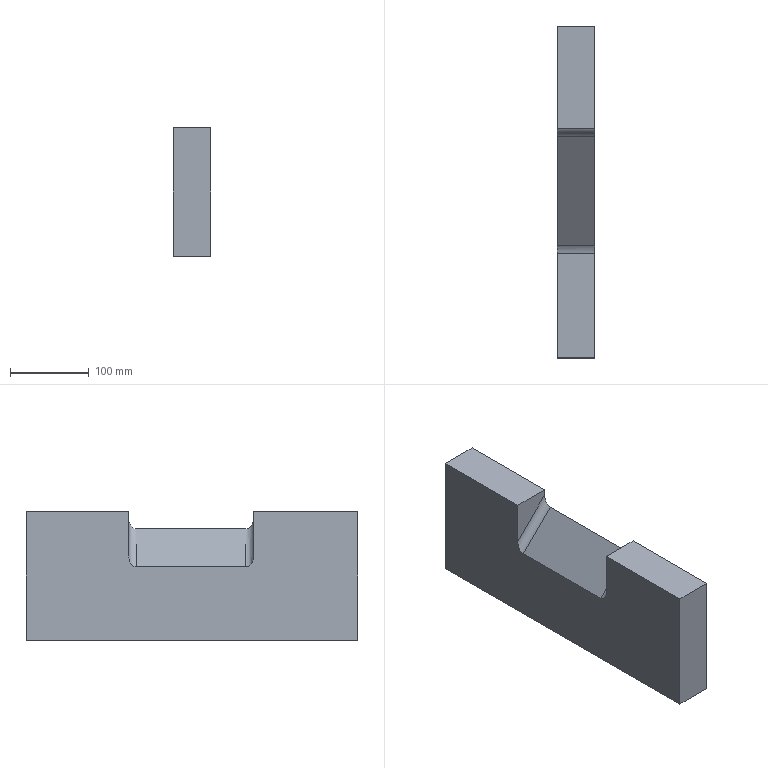Part | NX | features B2-2 2 | 1 solid | 18 faces | box 48 x 420 x 163 mm | volume 2923570 mm3 | plane 10 | cylinder 4 | cone 4 | commonest cylinder face diameters 14.506 x2 20 x2
STEP:
#1=CARTESIAN_POINT('',(2578.094,-927.317,711.716));
#2=VERTEX_POINT('',#1);
#3=CARTESIAN_POINT('',(2578.094,-788.927,711.716));
#4=VERTEX_POINT('',#3);
#5=CARTESIAN_POINT('',(2578.094,-859.122,711.716));
#6=DIRECTION('',(0.,-1.,0.));
#7=VECTOR('',#6,1000.);
#8=LINE('',#5,#7);
#9=EDGE_CURVE('',#2,#4,#8,.F.);
#10=ORIENTED_EDGE('',*,*,#9,.F.);
#11=CARTESIAN_POINT('',(2578.094,-937.317,725.858));
#12=VERTEX_POINT('',#11);
#13=CARTESIAN_POINT('',(2578.094,-927.317,725.858));
#14=DIRECTION('',(-1.,0.,0.));
#15=DIRECTION('',(0.,0.,-1.));
#16=AXIS2_PLACEMENT_3D('',#13,#14,#15);
#17=ELLIPSE('',#16,14.142,10.);
#18=EDGE_CURVE('',#2,#12,#17,.T.);
#19=ORIENTED_EDGE('',*,*,#18,.T.);
#20=CARTESIAN_POINT('',(2578.094,-937.317,733.716));
#21=VERTEX_POINT('',#20);
#22=CARTESIAN_POINT('',(2578.094,-937.317,768.716));
#23=DIRECTION('',(0.,0.,1.));
#24=VECTOR('',#23,1000.);
#25=LINE('',#22,#24);
#26=EDGE_CURVE('',#12,#21,#25,.T.);
#27=ORIENTED_EDGE('',*,*,#26,.T.);
#28=CARTESIAN_POINT('',(2578.094,-1069.122,733.716));
#29=VERTEX_POINT('',#28);
#30=CARTESIAN_POINT('',(2578.094,-859.122,733.716));
#31=DIRECTION('',(0.,1.,0.));
#32=VECTOR('',#31,1000.);
#33=LINE('',#30,#32);
#34=EDGE_CURVE('',#29,#21,#33,.T.);
#35=ORIENTED_EDGE('',*,*,#34,.F.);
#36=CARTESIAN_POINT('',(2578.094,-1069.122,570.716));
#37=VERTEX_POINT('',#36);
#38=CARTESIAN_POINT('',(2578.094,-1069.122,667.216));
#39=DIRECTION('',(0.,0.,-1.));
#40=VECTOR('',#39,1000.);
#41=LINE('',#38,#40);
#42=EDGE_CURVE('',#29,#37,#41,.T.);
#43=ORIENTED_EDGE('',*,*,#42,.T.);
#44=CARTESIAN_POINT('',(2578.094,-649.122,570.716));
#45=VERTEX_POINT('',#44);
#46=CARTESIAN_POINT('',(2578.094,0.,570.716));
#47=DIRECTION('',(0.,-1.,0.));
#48=VECTOR('',#47,1000.);
#49=LINE('',#46,#48);
#50=EDGE_CURVE('',#45,#37,#49,.T.);
#51=ORIENTED_EDGE('',*,*,#50,.F.);
#52=CARTESIAN_POINT('',(2578.094,-649.122,733.716));
#53=VERTEX_POINT('',#52);
#54=CARTESIAN_POINT('',(2578.094,-649.122,667.216));
#55=DIRECTION('',(0.,0.,1.));
#56=VECTOR('',#55,1000.);
#57=LINE('',#54,#56);
#58=EDGE_CURVE('',#45,#53,#57,.T.);
#59=ORIENTED_EDGE('',*,*,#58,.T.);
#60=CARTESIAN_POINT('',(2578.094,-778.927,733.716));
#61=VERTEX_POINT('',#60);
#62=CARTESIAN_POINT('',(2578.094,-859.122,733.716));
#63=DIRECTION('',(0.,1.,0.));
#64=VECTOR('',#63,1000.);
#65=LINE('',#62,#64);
#66=EDGE_CURVE('',#61,#53,#65,.T.);
#67=ORIENTED_EDGE('',*,*,#66,.F.);
#68=CARTESIAN_POINT('',(2578.094,-778.927,725.858));
#69=VERTEX_POINT('',#68);
#70=CARTESIAN_POINT('',(2578.094,-778.927,667.216));
#71=DIRECTION('',(0.,0.,1.));
#72=VECTOR('',#71,1000.);
#73=LINE('',#70,#72);
#74=EDGE_CURVE('',#69,#61,#73,.T.);
#75=ORIENTED_EDGE('',*,*,#74,.F.);
#76=CARTESIAN_POINT('',(2578.094,-788.927,725.858));
#77=DIRECTION('',(-1.,0.,0.));
#78=DIRECTION('',(0.,0.,1.));
#79=AXIS2_PLACEMENT_3D('',#76,#77,#78);
#80=ELLIPSE('',#79,14.142,10.);
#81=EDGE_CURVE('',#69,#4,#80,.T.);
#82=ORIENTED_EDGE('',*,*,#81,.T.);
#83=EDGE_LOOP('',(#10,#19,#27,#35,#43,#51,#59,#67,#75,#82));
#84=FACE_BOUND('',#83,.T.);
#85=CARTESIAN_POINT('',(2578.094,-859.122,667.216));
#86=DIRECTION('',(-1.,0.,0.));
#87=DIRECTION('',(0.,0.,-1.));
#88=AXIS2_PLACEMENT_3D('',#85,#86,#87);
#89=PLANE('',#88);
#90=ADVANCED_FACE('',(#84),#89,.F.);
#91=CARTESIAN_POINT('',(2530.094,-778.927,733.716));
#92=VERTEX_POINT('',#91);
#93=CARTESIAN_POINT('',(6910.188,-778.927,733.716));
#94=DIRECTION('',(-1.,0.,0.));
#95=VECTOR('',#94,1000.);
#96=LINE('',#93,#95);
#97=EDGE_CURVE('',#92,#61,#96,.F.);
#98=ORIENTED_EDGE('',*,*,#97,.T.);
#99=ORIENTED_EDGE('',*,*,#66,.T.);
#100=CARTESIAN_POINT('',(2530.094,-649.122,733.716));
#101=VERTEX_POINT('',#100);
#102=CARTESIAN_POINT('',(6910.188,-649.122,733.716));
#103=DIRECTION('',(-1.,0.,0.));
#104=VECTOR('',#103,1000.);
#105=LINE('',#102,#104);
#106=EDGE_CURVE('',#53,#101,#105,.T.);
#107=ORIENTED_EDGE('',*,*,#106,.T.);
#108=CARTESIAN_POINT('',(2530.094,-599.122,733.716));
#109=DIRECTION('',(0.,-1.,0.));
#110=VECTOR('',#109,1000.);
#111=LINE('',#108,#110);
#112=EDGE_CURVE('',#101,#92,#111,.T.);
#113=ORIENTED_EDGE('',*,*,#112,.T.);
#114=EDGE_LOOP('',(#98,#99,#107,#113));
#115=FACE_BOUND('',#114,.T.);
#116=CARTESIAN_POINT('',(6910.188,0.,733.716));
#117=DIRECTION('',(0.,0.,-1.));
#118=DIRECTION('',(1.,0.,0.));
#119=AXIS2_PLACEMENT_3D('',#116,#117,#118);
#120=PLANE('',#119);
#121=ADVANCED_FACE('',(#115),#120,.F.);
#122=CARTESIAN_POINT('',(2546.094,-669.122,570.716));
#123=VERTEX_POINT('',#122);
#124=CARTESIAN_POINT('',(2554.094,-669.122,570.716));
#125=DIRECTION('',(0.,0.,-1.));
#126=DIRECTION('',(-1.,0.,0.));
#127=AXIS2_PLACEMENT_3D('',#124,#125,#126);
#128=CIRCLE('',#127,8.);
#129=EDGE_CURVE('',#123,#123,#128,.T.);
#130=ORIENTED_EDGE('',*,*,#129,.F.);
#131=EDGE_LOOP('',(#130));
#132=FACE_BOUND('',#131,.T.);
#133=CARTESIAN_POINT('',(2546.094,-1049.122,570.716));
#134=VERTEX_POINT('',#133);
#135=CARTESIAN_POINT('',(2554.094,-1049.122,570.716));
#136=DIRECTION('',(0.,0.,-1.));
#137=DIRECTION('',(-1.,0.,0.));
#138=AXIS2_PLACEMENT_3D('',#135,#136,#137);
#139=CIRCLE('',#138,8.);
#140=EDGE_CURVE('',#134,#134,#139,.T.);
#141=ORIENTED_EDGE('',*,*,#140,.F.);
#142=EDGE_LOOP('',(#141));
#143=FACE_BOUND('',#142,.T.);
#144=CARTESIAN_POINT('',(2530.094,-1069.122,570.716));
#145=VERTEX_POINT('',#144);
#146=CARTESIAN_POINT('',(6910.188,-1069.122,570.716));
#147=DIRECTION('',(1.,0.,0.));
#148=VECTOR('',#147,1000.);
#149=LINE('',#146,#148);
#150=EDGE_CURVE('',#145,#37,#149,.T.);
#151=ORIENTED_EDGE('',*,*,#150,.F.);
#152=CARTESIAN_POINT('',(2530.094,-649.122,570.716));
#153=VERTEX_POINT('',#152);
#154=CARTESIAN_POINT('',(2530.094,-599.122,570.716));
#155=DIRECTION('',(0.,-1.,0.));
#156=VECTOR('',#155,1000.);
#157=LINE('',#154,#156);
#158=EDGE_CURVE('',#153,#145,#157,.T.);
#159=ORIENTED_EDGE('',*,*,#158,.F.);
#160=CARTESIAN_POINT('',(6910.188,-649.122,570.716));
#161=DIRECTION('',(-1.,0.,0.));
#162=VECTOR('',#161,1000.);
#163=LINE('',#160,#162);
#164=EDGE_CURVE('',#45,#153,#163,.T.);
#165=ORIENTED_EDGE('',*,*,#164,.F.);
#166=ORIENTED_EDGE('',*,*,#50,.T.);
#167=EDGE_LOOP('',(#151,#159,#165,#166));
#168=FACE_BOUND('',#167,.T.);
#169=CARTESIAN_POINT('',(6910.188,0.,570.716));
#170=DIRECTION('',(0.,0.,-1.));
#171=DIRECTION('',(1.,0.,0.));
#172=AXIS2_PLACEMENT_3D('',#169,#170,#171);
#173=PLANE('',#172);
#174=ADVANCED_FACE('',(#132,#143,#168),#173,.T.);
#175=ORIENTED_EDGE('',*,*,#34,.T.);
#176=CARTESIAN_POINT('',(2530.094,-937.317,733.716));
#177=VERTEX_POINT('',#176);
#178=CARTESIAN_POINT('',(6910.188,-937.317,733.716));
#179=DIRECTION('',(1.,0.,0.));
#180=VECTOR('',#179,1000.);
#181=LINE('',#178,#180);
#182=EDGE_CURVE('',#177,#21,#181,.T.);
#183=ORIENTED_EDGE('',*,*,#182,.F.);
#184=CARTESIAN_POINT('',(2530.094,-1069.122,733.716));
#185=VERTEX_POINT('',#184);
#186=CARTESIAN_POINT('',(2530.094,-599.122,733.716));
#187=DIRECTION('',(0.,-1.,0.));
#188=VECTOR('',#187,1000.);
#189=LINE('',#186,#188);
#190=EDGE_CURVE('',#177,#185,#189,.T.);
#191=ORIENTED_EDGE('',*,*,#190,.T.);
#192=CARTESIAN_POINT('',(6910.188,-1069.122,733.716));
#193=DIRECTION('',(1.,0.,0.));
#194=VECTOR('',#193,1000.);
#195=LINE('',#192,#194);
#196=EDGE_CURVE('',#185,#29,#195,.T.);
#197=ORIENTED_EDGE('',*,*,#196,.T.);
#198=EDGE_LOOP('',(#175,#183,#191,#197));
#199=FACE_BOUND('',#198,.T.);
#200=CARTESIAN_POINT('',(6910.188,0.,733.716));
#201=DIRECTION('',(0.,0.,-1.));
#202=DIRECTION('',(1.,0.,0.));
#203=AXIS2_PLACEMENT_3D('',#200,#201,#202);
#204=PLANE('',#203);
#205=ADVANCED_FACE('',(#199),#204,.F.);
#206=ORIENTED_EDGE('',*,*,#196,.F.);
#207=CARTESIAN_POINT('',(2530.094,-1069.122,600.716));
#208=DIRECTION('',(0.,0.,1.));
#209=VECTOR('',#208,1000.);
#210=LINE('',#207,#209);
#211=EDGE_CURVE('',#145,#185,#210,.T.);
#212=ORIENTED_EDGE('',*,*,#211,.F.);
#213=ORIENTED_EDGE('',*,*,#150,.T.);
#214=ORIENTED_EDGE('',*,*,#42,.F.);
#215=EDGE_LOOP('',(#206,#212,#213,#214));
#216=FACE_BOUND('',#215,.T.);
#217=CARTESIAN_POINT('',(2530.094,-1069.122,600.716));
#218=DIRECTION('',(0.,1.,0.));
#219=DIRECTION('',(1.,0.,0.));
#220=AXIS2_PLACEMENT_3D('',#217,#218,#219);
#221=PLANE('',#220);
#222=ADVANCED_FACE('',(#216),#221,.F.);
#223=ORIENTED_EDGE('',*,*,#164,.T.);
#224=CARTESIAN_POINT('',(2530.094,-649.122,600.716));
#225=DIRECTION('',(0.,0.,1.));
#226=VECTOR('',#225,1000.);
#227=LINE('',#224,#226);
#228=EDGE_CURVE('',#153,#101,#227,.T.);
#229=ORIENTED_EDGE('',*,*,#228,.T.);
#230=ORIENTED_EDGE('',*,*,#106,.F.);
#231=ORIENTED_EDGE('',*,*,#58,.F.);
#232=EDGE_LOOP('',(#223,#229,#230,#231));
#233=FACE_BOUND('',#232,.T.);
#234=CARTESIAN_POINT('',(4655.094,-649.122,600.716));
#235=DIRECTION('',(0.,-1.,0.));
#236=DIRECTION('',(0.,0.,-1.));
#237=AXIS2_PLACEMENT_3D('',#234,#235,#236);
#238=PLANE('',#237);
#239=ADVANCED_FACE('',(#233),#238,.F.);
#240=CARTESIAN_POINT('',(2530.094,-937.317,677.858));
#241=VERTEX_POINT('',#240);
#242=CARTESIAN_POINT('',(2530.094,-937.317,600.716));
#243=DIRECTION('',(0.,0.,1.));
#244=VECTOR('',#243,1000.);
#245=LINE('',#242,#244);
#246=EDGE_CURVE('',#177,#241,#245,.F.);
#247=ORIENTED_EDGE('',*,*,#246,.T.);
#248=CARTESIAN_POINT('',(2530.094,-927.317,663.716));
#249=VERTEX_POINT('',#248);
#250=CARTESIAN_POINT('',(2530.094,-927.317,677.858));
#251=DIRECTION('',(1.,0.,0.));
#252=DIRECTION('',(0.,0.,-1.));
#253=AXIS2_PLACEMENT_3D('',#250,#251,#252);
#254=ELLIPSE('',#253,14.142,10.);
#255=EDGE_CURVE('',#241,#249,#254,.T.);
#256=ORIENTED_EDGE('',*,*,#255,.T.);
#257=CARTESIAN_POINT('',(2530.094,-788.927,663.716));
#258=VERTEX_POINT('',#257);
#259=CARTESIAN_POINT('',(2530.094,0.,663.716));
#260=DIRECTION('',(0.,-1.,0.));
#261=VECTOR('',#260,1000.);
#262=LINE('',#259,#261);
#263=EDGE_CURVE('',#249,#258,#262,.F.);
#264=ORIENTED_EDGE('',*,*,#263,.T.);
#265=CARTESIAN_POINT('',(2530.094,-778.927,677.858));
#266=VERTEX_POINT('',#265);
#267=CARTESIAN_POINT('',(2530.094,-788.927,677.858));
#268=DIRECTION('',(1.,0.,0.));
#269=DIRECTION('',(0.,0.,1.));
#270=AXIS2_PLACEMENT_3D('',#267,#268,#269);
#271=ELLIPSE('',#270,14.142,10.);
#272=EDGE_CURVE('',#258,#266,#271,.T.);
#273=ORIENTED_EDGE('',*,*,#272,.T.);
#274=CARTESIAN_POINT('',(2530.094,-778.927,600.716));
#275=DIRECTION('',(0.,0.,-1.));
#276=VECTOR('',#275,1000.);
#277=LINE('',#274,#276);
#278=EDGE_CURVE('',#92,#266,#277,.T.);
#279=ORIENTED_EDGE('',*,*,#278,.F.);
#280=ORIENTED_EDGE('',*,*,#112,.F.);
#281=ORIENTED_EDGE('',*,*,#228,.F.);
#282=ORIENTED_EDGE('',*,*,#158,.T.);
#283=ORIENTED_EDGE('',*,*,#211,.T.);
#284=ORIENTED_EDGE('',*,*,#190,.F.);
#285=EDGE_LOOP('',(#247,#256,#264,#273,#279,#280,#281,#282,#283,#284));
#286=FACE_BOUND('',#285,.T.);
#287=CARTESIAN_POINT('',(2530.094,-599.122,600.716));
#288=DIRECTION('',(1.,0.,0.));
#289=DIRECTION('',(0.,0.,1.));
#290=AXIS2_PLACEMENT_3D('',#287,#288,#289);
#291=PLANE('',#290);
#292=ADVANCED_FACE('',(#286),#291,.F.);
#293=ORIENTED_EDGE('',*,*,#278,.T.);
#294=CARTESIAN_POINT('',(2571.023,-778.927,718.787));
#295=DIRECTION('',(-0.7071,0.,-0.7071));
#296=VECTOR('',#295,1000.);
#297=LINE('',#294,#296);
#298=EDGE_CURVE('',#266,#69,#297,.F.);
#299=ORIENTED_EDGE('',*,*,#298,.T.);
#300=ORIENTED_EDGE('',*,*,#74,.T.);
#301=ORIENTED_EDGE('',*,*,#97,.F.);
#302=EDGE_LOOP('',(#293,#299,#300,#301));
#303=FACE_BOUND('',#302,.T.);
#304=CARTESIAN_POINT('',(2530.509,-778.927,768.716));
#305=DIRECTION('',(0.,-1.,0.));
#306=DIRECTION('',(0.,0.,-1.));
#307=AXIS2_PLACEMENT_3D('',#304,#305,#306);
#308=PLANE('',#307);
#309=ADVANCED_FACE('',(#303),#308,.T.);
#310=ORIENTED_EDGE('',*,*,#26,.F.);
#311=CARTESIAN_POINT('',(2523.023,-937.317,670.787));
#312=DIRECTION('',(0.7071,0.,0.7071));
#313=VECTOR('',#312,1000.);
#314=LINE('',#311,#313);
#315=EDGE_CURVE('',#12,#241,#314,.F.);
#316=ORIENTED_EDGE('',*,*,#315,.T.);
#317=ORIENTED_EDGE('',*,*,#246,.F.);
#318=ORIENTED_EDGE('',*,*,#182,.T.);
#319=EDGE_LOOP('',(#310,#316,#317,#318));
#320=FACE_BOUND('',#319,.T.);
#321=CARTESIAN_POINT('',(2530.509,-937.317,768.716));
#322=DIRECTION('',(0.,1.,0.));
#323=DIRECTION('',(0.,0.,1.));
#324=AXIS2_PLACEMENT_3D('',#321,#322,#323);
#325=PLANE('',#324);
#326=ADVANCED_FACE('',(#320),#325,.T.);
#327=ORIENTED_EDGE('',*,*,#9,.T.);
#328=CARTESIAN_POINT('',(2530.094,-788.927,663.716));
#329=DIRECTION('',(0.7071,0.,0.7071));
#330=VECTOR('',#329,1000.);
#331=LINE('',#328,#330);
#332=EDGE_CURVE('',#4,#258,#331,.F.);
#333=ORIENTED_EDGE('',*,*,#332,.T.);
#334=ORIENTED_EDGE('',*,*,#263,.F.);
#335=CARTESIAN_POINT('',(2578.094,-927.317,711.716));
#336=DIRECTION('',(-0.7071,0.,-0.7071));
#337=VECTOR('',#336,1000.);
#338=LINE('',#335,#337);
#339=EDGE_CURVE('',#249,#2,#338,.F.);
#340=ORIENTED_EDGE('',*,*,#339,.T.);
#341=EDGE_LOOP('',(#327,#333,#334,#340));
#342=FACE_BOUND('',#341,.T.);
#343=CARTESIAN_POINT('',(2580.094,0.,713.716));
#344=DIRECTION('',(0.7071,0.,-0.7071));
#345=DIRECTION('',(0.,-1.,0.));
#346=AXIS2_PLACEMENT_3D('',#343,#344,#345);
#347=PLANE('',#346);
#348=ADVANCED_FACE('',(#342),#347,.F.);
#349=ORIENTED_EDGE('',*,*,#272,.F.);
#350=ORIENTED_EDGE('',*,*,#332,.F.);
#351=ORIENTED_EDGE('',*,*,#81,.F.);
#352=ORIENTED_EDGE('',*,*,#298,.F.);
#353=EDGE_LOOP('',(#349,#350,#351,#352));
#354=FACE_BOUND('',#353,.T.);
#355=CARTESIAN_POINT('',(2575.73,-788.927,723.495));
#356=DIRECTION('',(0.7071,0.,0.7071));
#357=DIRECTION('',(0.7071,0.,-0.7071));
#358=AXIS2_PLACEMENT_3D('',#355,#356,#357);
#359=CYLINDRICAL_SURFACE('',#358,10.);
#360=ADVANCED_FACE('',(#354),#359,.F.);
#361=ORIENTED_EDGE('',*,*,#18,.F.);
#362=ORIENTED_EDGE('',*,*,#339,.F.);
#363=ORIENTED_EDGE('',*,*,#255,.F.);
#364=ORIENTED_EDGE('',*,*,#315,.F.);
#365=EDGE_LOOP('',(#361,#362,#363,#364));
#366=FACE_BOUND('',#365,.T.);
#367=CARTESIAN_POINT('',(2575.73,-927.317,723.495));
#368=DIRECTION('',(-0.7071,0.,-0.7071));
#369=DIRECTION('',(-0.7071,0.,0.7071));
#370=AXIS2_PLACEMENT_3D('',#367,#368,#369);
#371=CYLINDRICAL_SURFACE('',#370,10.);
#372=ADVANCED_FACE('',(#366),#371,.F.);
#373=CARTESIAN_POINT('',(2546.841,-1049.122,571.463));
#374=VERTEX_POINT('',#373);
#375=CARTESIAN_POINT('',(2554.094,-1049.122,571.463));
#376=DIRECTION('',(0.,0.,-1.));
#377=DIRECTION('',(-1.,0.,0.));
#378=AXIS2_PLACEMENT_3D('',#375,#376,#377);
#379=CIRCLE('',#378,7.253);
#380=EDGE_CURVE('',#374,#374,#379,.F.);
#381=ORIENTED_EDGE('',*,*,#380,.F.);
#382=EDGE_LOOP('',(#381));
#383=FACE_BOUND('',#382,.T.);
#384=CARTESIAN_POINT('',(2546.841,-1049.122,615.713));
#385=VERTEX_POINT('',#384);
#386=CARTESIAN_POINT('',(2554.094,-1049.122,615.713));
#387=DIRECTION('',(0.,0.,-1.));
#388=DIRECTION('',(-1.,0.,0.));
#389=AXIS2_PLACEMENT_3D('',#386,#387,#388);
#390=CIRCLE('',#389,7.253);
#391=EDGE_CURVE('',#385,#385,#390,.F.);
#392=ORIENTED_EDGE('',*,*,#391,.T.);
#393=EDGE_LOOP('',(#392));
#394=FACE_BOUND('',#393,.T.);
#395=CARTESIAN_POINT('',(2554.094,-1049.122,622.966));
#396=DIRECTION('',(0.,0.,-1.));
#397=DIRECTION('',(-1.,0.,0.));
#398=AXIS2_PLACEMENT_3D('',#395,#396,#397);
#399=CYLINDRICAL_SURFACE('',#398,7.253);
#400=ADVANCED_FACE('',(#383,#394),#399,.F.);
#401=CARTESIAN_POINT('',(2554.094,-1049.122,622.966));
#402=VERTEX_POINT('',#401);
#403=VERTEX_LOOP('',#402);
#404=FACE_BOUND('',#403,.T.);
#405=ORIENTED_EDGE('',*,*,#391,.F.);
#406=EDGE_LOOP('',(#405));
#407=FACE_BOUND('',#406,.T.);
#408=CARTESIAN_POINT('',(2554.094,-1049.122,615.716));
#409=DIRECTION('',(0.,0.,-1.));
#410=DIRECTION('',(-1.,0.,0.));
#411=AXIS2_PLACEMENT_3D('',#408,#409,#410);
#412=CONICAL_SURFACE('',#411,7.25,0.7854);
#413=ADVANCED_FACE('',(#404,#407),#412,.F.);
#414=ORIENTED_EDGE('',*,*,#380,.T.);
#415=EDGE_LOOP('',(#414));
#416=FACE_BOUND('',#415,.T.);
#417=ORIENTED_EDGE('',*,*,#140,.T.);
#418=EDGE_LOOP('',(#417));
#419=FACE_BOUND('',#418,.T.);
#420=CARTESIAN_POINT('',(2554.094,-1049.122,570.716));
#421=DIRECTION('',(0.,0.,-1.));
#422=DIRECTION('',(-1.,0.,0.));
#423=AXIS2_PLACEMENT_3D('',#420,#421,#422);
#424=CONICAL_SURFACE('',#423,8.,0.7854);
#425=ADVANCED_FACE('',(#416,#419),#424,.F.);
#426=CARTESIAN_POINT('',(2546.841,-669.122,571.463));
#427=VERTEX_POINT('',#426);
#428=CARTESIAN_POINT('',(2554.094,-669.122,571.463));
#429=DIRECTION('',(0.,0.,-1.));
#430=DIRECTION('',(-1.,0.,0.));
#431=AXIS2_PLACEMENT_3D('',#428,#429,#430);
#432=CIRCLE('',#431,7.253);
#433=EDGE_CURVE('',#427,#427,#432,.F.);
#434=ORIENTED_EDGE('',*,*,#433,.F.);
#435=EDGE_LOOP('',(#434));
#436=FACE_BOUND('',#435,.T.);
#437=CARTESIAN_POINT('',(2546.841,-669.122,615.713));
#438=VERTEX_POINT('',#437);
#439=CARTESIAN_POINT('',(2554.094,-669.122,615.713));
#440=DIRECTION('',(0.,0.,-1.));
#441=DIRECTION('',(-1.,0.,0.));
#442=AXIS2_PLACEMENT_3D('',#439,#440,#441);
#443=CIRCLE('',#442,7.253);
#444=EDGE_CURVE('',#438,#438,#443,.F.);
#445=ORIENTED_EDGE('',*,*,#444,.T.);
#446=EDGE_LOOP('',(#445));
#447=FACE_BOUND('',#446,.T.);
#448=CARTESIAN_POINT('',(2554.094,-669.122,622.966));
#449=DIRECTION('',(0.,0.,-1.));
#450=DIRECTION('',(-1.,0.,0.));
#451=AXIS2_PLACEMENT_3D('',#448,#449,#450);
#452=CYLINDRICAL_SURFACE('',#451,7.253);
#453=ADVANCED_FACE('',(#436,#447),#452,.F.);
#454=CARTESIAN_POINT('',(2554.094,-669.122,622.966));
#455=VERTEX_POINT('',#454);
#456=VERTEX_LOOP('',#455);
#457=FACE_BOUND('',#456,.T.);
#458=ORIENTED_EDGE('',*,*,#444,.F.);
#459=EDGE_LOOP('',(#458));
#460=FACE_BOUND('',#459,.T.);
#461=CARTESIAN_POINT('',(2554.094,-669.122,615.716));
#462=DIRECTION('',(0.,0.,-1.));
#463=DIRECTION('',(-1.,0.,0.));
#464=AXIS2_PLACEMENT_3D('',#461,#462,#463);
#465=CONICAL_SURFACE('',#464,7.25,0.7854);
#466=ADVANCED_FACE('',(#457,#460),#465,.F.);
#467=ORIENTED_EDGE('',*,*,#433,.T.);
#468=EDGE_LOOP('',(#467));
#469=FACE_BOUND('',#468,.T.);
#470=ORIENTED_EDGE('',*,*,#129,.T.);
#471=EDGE_LOOP('',(#470));
#472=FACE_BOUND('',#471,.T.);
#473=CARTESIAN_POINT('',(2554.094,-669.122,570.716));
#474=DIRECTION('',(0.,0.,-1.));
#475=DIRECTION('',(-1.,0.,0.));
#476=AXIS2_PLACEMENT_3D('',#473,#474,#475);
#477=CONICAL_SURFACE('',#476,8.,0.7854);
#478=ADVANCED_FACE('',(#469,#472),#477,.F.);
#479=CLOSED_SHELL('',(#90,#121,#174,#205,#222,#239,#292,#309,#326,#348,#360,#372,#400,#413,#425,#453,#466,#478));
#480=MANIFOLD_SOLID_BREP('',#479);
#481=(LENGTH_UNIT()NAMED_UNIT(*)SI_UNIT(.MILLI.,.METRE.));
#482=UNCERTAINTY_MEASURE_WITH_UNIT(LENGTH_MEASURE(0.00001),#481,'','');
#483=(NAMED_UNIT(*)PLANE_ANGLE_UNIT()SI_UNIT($,.RADIAN.));
#484=(NAMED_UNIT(*)SI_UNIT($,.STERADIAN.)SOLID_ANGLE_UNIT());
#485=(GEOMETRIC_REPRESENTATION_CONTEXT(3)GLOBAL_UNCERTAINTY_ASSIGNED_CONTEXT((#482))GLOBAL_UNIT_ASSIGNED_CONTEXT((#481,#483,#484))REPRESENTATION_CONTEXT('',''));
#486=ADVANCED_BREP_SHAPE_REPRESENTATION('',(#480),#485);